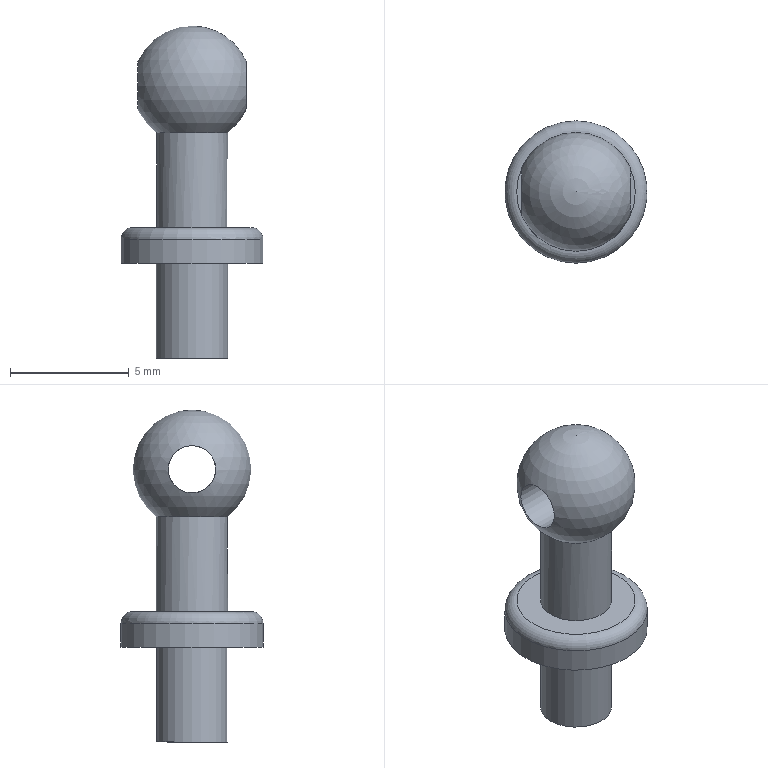Part | STEP file | 1-33.1 | 1 solid | 9 faces | box 6 x 6 x 14 mm | volume 146.542 mm3 | cylinder 4 | plane 3 | sphere 1 | torus 1 | commonest cylinder face diameters 3 x2 2 x1 6 x1
STEP:
#1=CARTESIAN_POINT('',(0.,0.,0.));
#2=DIRECTION('',(0.,0.,1.));
#3=DIRECTION('',(1.,0.,0.));
#4=AXIS2_PLACEMENT_3D('',#1,#2,#3);
#5=CARTESIAN_POINT('',(0.,1.5,-6.));
#6=VERTEX_POINT('',#5);
#7=CARTESIAN_POINT('',(0.,0.,-6.));
#8=DIRECTION('',(0.,0.,-1.));
#9=DIRECTION('',(0.,1.,0.));
#10=AXIS2_PLACEMENT_3D('',#7,#8,#9);
#11=CIRCLE('',#10,1.5);
#12=CARTESIAN_POINT('',(0.,0.,0.));
#13=DIRECTION('',(0.,0.,-1.));
#14=DIRECTION('',(0.,1.,0.));
#15=AXIS2_PLACEMENT_3D('',#12,#13,#14);
#16=CYLINDRICAL_SURFACE('',#15,1.5);
#17=CARTESIAN_POINT('',(0.,6.));
#18=DIRECTION('',(1.,0.));
#19=VECTOR('',#18,1.);
#20=LINE('',#17,#19);
#21=(GEOMETRIC_REPRESENTATION_CONTEXT(2)PARAMETRIC_REPRESENTATION_CONTEXT()REPRESENTATION_CONTEXT('',''));
#22=DEFINITIONAL_REPRESENTATION('',(#20),#21);
#23=PCURVE('',#16,#22);
#24=CARTESIAN_POINT('',(0.,-0.8038,-6.));
#25=DIRECTION('',(0.,0.,-1.));
#26=DIRECTION('',(0.,1.,0.));
#27=AXIS2_PLACEMENT_3D('',#24,#25,#26);
#28=PLANE('',#27);
#29=CARTESIAN_POINT('',(0.8038,0.));
#30=DIRECTION('',(1.,0.));
#31=AXIS2_PLACEMENT_2D('',#29,#30);
#32=CIRCLE('',#31,1.5);
#33=(GEOMETRIC_REPRESENTATION_CONTEXT(2)PARAMETRIC_REPRESENTATION_CONTEXT()REPRESENTATION_CONTEXT('',''));
#34=DEFINITIONAL_REPRESENTATION('',(#32),#33);
#35=PCURVE('',#28,#34);
#36=SURFACE_CURVE('',#11,(#23,#35),.PCURVE_S1.);
#37=EDGE_CURVE('',#6,#6,#36,.T.);
#38=ORIENTED_EDGE('',*,*,#37,.F.);
#39=CARTESIAN_POINT('',(0.,1.5,-2.));
#40=VERTEX_POINT('',#39);
#41=CARTESIAN_POINT('',(0.,1.5,-2.));
#42=DIRECTION('',(0.,0.,-1.));
#43=VECTOR('',#42,1.);
#44=LINE('',#41,#43);
#45=CARTESIAN_POINT('',(0.,2.));
#46=DIRECTION('',(0.,1.));
#47=VECTOR('',#46,1.);
#48=LINE('',#45,#47);
#49=(GEOMETRIC_REPRESENTATION_CONTEXT(2)PARAMETRIC_REPRESENTATION_CONTEXT()REPRESENTATION_CONTEXT('',''));
#50=DEFINITIONAL_REPRESENTATION('',(#48),#49);
#51=PCURVE('',#16,#50);
#52=CARTESIAN_POINT('',(6.283,2.));
#53=DIRECTION('',(0.,1.));
#54=VECTOR('',#53,1.);
#55=LINE('',#52,#54);
#56=(GEOMETRIC_REPRESENTATION_CONTEXT(2)PARAMETRIC_REPRESENTATION_CONTEXT()REPRESENTATION_CONTEXT('',''));
#57=DEFINITIONAL_REPRESENTATION('',(#55),#56);
#58=PCURVE('',#16,#57);
#59=SEAM_CURVE('',#44,(#51,#58),.PCURVE_S1.);
#60=EDGE_CURVE('',#40,#6,#59,.T.);
#61=ORIENTED_EDGE('',*,*,#60,.F.);
#62=CARTESIAN_POINT('',(1.5,0.,-2.));
#63=VERTEX_POINT('',#62);
#64=CARTESIAN_POINT('',(0.,0.,-2.));
#65=DIRECTION('',(0.,0.,-1.));
#66=DIRECTION('',(0.,1.,0.));
#67=AXIS2_PLACEMENT_3D('',#64,#65,#66);
#68=CIRCLE('',#67,1.5);
#69=CARTESIAN_POINT('',(0.,2.));
#70=DIRECTION('',(1.,0.));
#71=VECTOR('',#70,1.);
#72=LINE('',#69,#71);
#73=(GEOMETRIC_REPRESENTATION_CONTEXT(2)PARAMETRIC_REPRESENTATION_CONTEXT()REPRESENTATION_CONTEXT('',''));
#74=DEFINITIONAL_REPRESENTATION('',(#72),#73);
#75=PCURVE('',#16,#74);
#76=CARTESIAN_POINT('',(0.,0.,0.));
#77=DIRECTION('',(0.,0.,1.));
#78=DIRECTION('',(1.,0.,0.));
#79=AXIS2_PLACEMENT_3D('',#76,#77,#78);
#80=SPHERICAL_SURFACE('',#79,2.5);
#81=CARTESIAN_POINT('',(1.571,-0.9273));
#82=DIRECTION('',(-1.,0.));
#83=VECTOR('',#82,1.);
#84=LINE('',#81,#83);
#85=(GEOMETRIC_REPRESENTATION_CONTEXT(2)PARAMETRIC_REPRESENTATION_CONTEXT()REPRESENTATION_CONTEXT('',''));
#86=DEFINITIONAL_REPRESENTATION('',(#84),#85);
#87=PCURVE('',#80,#86);
#88=SURFACE_CURVE('',#68,(#75,#87),.PCURVE_S1.);
#89=EDGE_CURVE('',#40,#63,#88,.T.);
#90=ORIENTED_EDGE('',*,*,#89,.T.);
#91=CARTESIAN_POINT('',(0.,0.,-2.));
#92=DIRECTION('',(0.,0.,-1.));
#93=DIRECTION('',(1.,0.,0.));
#94=AXIS2_PLACEMENT_3D('',#91,#92,#93);
#95=CIRCLE('',#94,1.5);
#96=CARTESIAN_POINT('',(1.571,2.));
#97=DIRECTION('',(1.,0.));
#98=VECTOR('',#97,1.);
#99=LINE('',#96,#98);
#100=(GEOMETRIC_REPRESENTATION_CONTEXT(2)PARAMETRIC_REPRESENTATION_CONTEXT()REPRESENTATION_CONTEXT('',''));
#101=DEFINITIONAL_REPRESENTATION('',(#99),#100);
#102=PCURVE('',#16,#101);
#103=CARTESIAN_POINT('',(6.283,-0.9273));
#104=DIRECTION('',(-1.,0.));
#105=VECTOR('',#104,1.);
#106=LINE('',#103,#105);
#107=(GEOMETRIC_REPRESENTATION_CONTEXT(2)PARAMETRIC_REPRESENTATION_CONTEXT()REPRESENTATION_CONTEXT('',''));
#108=DEFINITIONAL_REPRESENTATION('',(#106),#107);
#109=PCURVE('',#80,#108);
#110=SURFACE_CURVE('',#95,(#102,#109),.PCURVE_S1.);
#111=EDGE_CURVE('',#63,#40,#110,.T.);
#112=ORIENTED_EDGE('',*,*,#111,.T.);
#113=ORIENTED_EDGE('',*,*,#60,.T.);
#114=EDGE_LOOP('',(#38,#61,#90,#112,#113));
#115=FACE_BOUND('',#114,.T.);
#116=ADVANCED_FACE('',(#115),#16,.T.);
#117=CARTESIAN_POINT('',(0.,3.,-7.5));
#118=VERTEX_POINT('',#117);
#119=CARTESIAN_POINT('',(0.,0.,-7.5));
#120=DIRECTION('',(0.,0.,-1.));
#121=DIRECTION('',(0.,1.,0.));
#122=AXIS2_PLACEMENT_3D('',#119,#120,#121);
#123=CIRCLE('',#122,3.);
#124=CARTESIAN_POINT('',(0.,-0.8038,-7.5));
#125=DIRECTION('',(0.,0.,-1.));
#126=DIRECTION('',(0.,1.,0.));
#127=AXIS2_PLACEMENT_3D('',#124,#125,#126);
#128=PLANE('',#127);
#129=CARTESIAN_POINT('',(0.8038,0.));
#130=DIRECTION('',(1.,0.));
#131=AXIS2_PLACEMENT_2D('',#129,#130);
#132=CIRCLE('',#131,3.);
#133=(GEOMETRIC_REPRESENTATION_CONTEXT(2)PARAMETRIC_REPRESENTATION_CONTEXT()REPRESENTATION_CONTEXT('',''));
#134=DEFINITIONAL_REPRESENTATION('',(#132),#133);
#135=PCURVE('',#128,#134);
#136=CARTESIAN_POINT('',(0.,0.,-6.));
#137=DIRECTION('',(0.,0.,-1.));
#138=DIRECTION('',(0.,1.,0.));
#139=AXIS2_PLACEMENT_3D('',#136,#137,#138);
#140=CYLINDRICAL_SURFACE('',#139,3.);
#141=CARTESIAN_POINT('',(0.,1.5));
#142=DIRECTION('',(1.,0.));
#143=VECTOR('',#142,1.);
#144=LINE('',#141,#143);
#145=(GEOMETRIC_REPRESENTATION_CONTEXT(2)PARAMETRIC_REPRESENTATION_CONTEXT()REPRESENTATION_CONTEXT('',''));
#146=DEFINITIONAL_REPRESENTATION('',(#144),#145);
#147=PCURVE('',#140,#146);
#148=SURFACE_CURVE('',#123,(#135,#147),.PCURVE_S1.);
#149=EDGE_CURVE('',#118,#118,#148,.T.);
#150=ORIENTED_EDGE('',*,*,#149,.T.);
#151=EDGE_LOOP('',(#150));
#152=FACE_BOUND('',#151,.T.);
#153=CARTESIAN_POINT('',(1.5,0.,-7.5));
#154=VERTEX_POINT('',#153);
#155=CARTESIAN_POINT('',(0.,0.,-7.5));
#156=DIRECTION('',(0.,0.,-1.));
#157=DIRECTION('',(1.,0.,0.));
#158=AXIS2_PLACEMENT_3D('',#155,#156,#157);
#159=CIRCLE('',#158,1.5);
#160=CARTESIAN_POINT('',(0.8038,0.));
#161=DIRECTION('',(0.,1.));
#162=AXIS2_PLACEMENT_2D('',#160,#161);
#163=CIRCLE('',#162,1.5);
#164=(GEOMETRIC_REPRESENTATION_CONTEXT(2)PARAMETRIC_REPRESENTATION_CONTEXT()REPRESENTATION_CONTEXT('',''));
#165=DEFINITIONAL_REPRESENTATION('',(#163),#164);
#166=PCURVE('',#128,#165);
#167=CARTESIAN_POINT('',(0.,0.,-7.5));
#168=DIRECTION('',(0.,0.,-1.));
#169=DIRECTION('',(1.,0.,0.));
#170=AXIS2_PLACEMENT_3D('',#167,#168,#169);
#171=CYLINDRICAL_SURFACE('',#170,1.5);
#172=CARTESIAN_POINT('',(0.,0.));
#173=DIRECTION('',(1.,0.));
#174=VECTOR('',#173,1.);
#175=LINE('',#172,#174);
#176=(GEOMETRIC_REPRESENTATION_CONTEXT(2)PARAMETRIC_REPRESENTATION_CONTEXT()REPRESENTATION_CONTEXT('',''));
#177=DEFINITIONAL_REPRESENTATION('',(#175),#176);
#178=PCURVE('',#171,#177);
#179=SURFACE_CURVE('',#159,(#166,#178),.PCURVE_S1.);
#180=EDGE_CURVE('',#154,#154,#179,.T.);
#181=ORIENTED_EDGE('',*,*,#180,.F.);
#182=EDGE_LOOP('',(#181));
#183=FACE_BOUND('',#182,.T.);
#184=ADVANCED_FACE('',(#152,#183),#128,.T.);
#185=ORIENTED_EDGE('',*,*,#180,.T.);
#186=CARTESIAN_POINT('',(1.5,0.,-11.5));
#187=VERTEX_POINT('',#186);
#188=CARTESIAN_POINT('',(1.5,0.,-7.5));
#189=DIRECTION('',(0.,0.,-1.));
#190=VECTOR('',#189,1.);
#191=LINE('',#188,#190);
#192=CARTESIAN_POINT('',(6.283,0.));
#193=DIRECTION('',(0.,1.));
#194=VECTOR('',#193,1.);
#195=LINE('',#192,#194);
#196=(GEOMETRIC_REPRESENTATION_CONTEXT(2)PARAMETRIC_REPRESENTATION_CONTEXT()REPRESENTATION_CONTEXT('',''));
#197=DEFINITIONAL_REPRESENTATION('',(#195),#196);
#198=PCURVE('',#171,#197);
#199=CARTESIAN_POINT('',(0.,0.));
#200=DIRECTION('',(0.,1.));
#201=VECTOR('',#200,1.);
#202=LINE('',#199,#201);
#203=(GEOMETRIC_REPRESENTATION_CONTEXT(2)PARAMETRIC_REPRESENTATION_CONTEXT()REPRESENTATION_CONTEXT('',''));
#204=DEFINITIONAL_REPRESENTATION('',(#202),#203);
#205=PCURVE('',#171,#204);
#206=SEAM_CURVE('',#191,(#198,#205),.PCURVE_S1.);
#207=EDGE_CURVE('',#154,#187,#206,.T.);
#208=ORIENTED_EDGE('',*,*,#207,.T.);
#209=CARTESIAN_POINT('',(0.,0.,-11.5));
#210=DIRECTION('',(0.,0.,-1.));
#211=DIRECTION('',(1.,0.,0.));
#212=AXIS2_PLACEMENT_3D('',#209,#210,#211);
#213=CIRCLE('',#212,1.5);
#214=CARTESIAN_POINT('',(0.,4.));
#215=DIRECTION('',(1.,0.));
#216=VECTOR('',#215,1.);
#217=LINE('',#214,#216);
#218=(GEOMETRIC_REPRESENTATION_CONTEXT(2)PARAMETRIC_REPRESENTATION_CONTEXT()REPRESENTATION_CONTEXT('',''));
#219=DEFINITIONAL_REPRESENTATION('',(#217),#218);
#220=PCURVE('',#171,#219);
#221=CARTESIAN_POINT('',(-0.4019,0.,-11.5));
#222=DIRECTION('',(0.,0.,-1.));
#223=DIRECTION('',(1.,0.,0.));
#224=AXIS2_PLACEMENT_3D('',#221,#222,#223);
#225=PLANE('',#224);
#226=CARTESIAN_POINT('',(0.4019,0.));
#227=DIRECTION('',(1.,0.));
#228=AXIS2_PLACEMENT_2D('',#226,#227);
#229=CIRCLE('',#228,1.5);
#230=(GEOMETRIC_REPRESENTATION_CONTEXT(2)PARAMETRIC_REPRESENTATION_CONTEXT()REPRESENTATION_CONTEXT('',''));
#231=DEFINITIONAL_REPRESENTATION('',(#229),#230);
#232=PCURVE('',#225,#231);
#233=SURFACE_CURVE('',#213,(#220,#232),.PCURVE_S1.);
#234=EDGE_CURVE('',#187,#187,#233,.T.);
#235=ORIENTED_EDGE('',*,*,#234,.F.);
#236=ORIENTED_EDGE('',*,*,#207,.F.);
#237=EDGE_LOOP('',(#185,#208,#235,#236));
#238=FACE_BOUND('',#237,.T.);
#239=ADVANCED_FACE('',(#238),#171,.T.);
#240=ORIENTED_EDGE('',*,*,#234,.T.);
#241=EDGE_LOOP('',(#240));
#242=FACE_BOUND('',#241,.T.);
#243=ADVANCED_FACE('',(#242),#225,.T.);
#244=CARTESIAN_POINT('',(2.291,0.,1.));
#245=VERTEX_POINT('',#244);
#246=CARTESIAN_POINT('',(0.,0.,2.5));
#247=VERTEX_POINT('',#246);
#248=CARTESIAN_POINT('',(0.,0.,0.));
#249=DIRECTION('',(0.,-1.,0.));
#250=DIRECTION('',(0.9165,0.,0.4));
#251=AXIS2_PLACEMENT_3D('',#248,#249,#250);
#252=CIRCLE('',#251,2.5);
#253=CARTESIAN_POINT('',(0.,0.4115));
#254=CARTESIAN_POINT('',(0.,0.4291));
#255=CARTESIAN_POINT('',(0.,0.4642));
#256=CARTESIAN_POINT('',(0.,0.5169));
#257=CARTESIAN_POINT('',(0.,0.5696));
#258=CARTESIAN_POINT('',(0.,0.6223));
#259=CARTESIAN_POINT('',(0.,0.675));
#260=CARTESIAN_POINT('',(0.,0.7277));
#261=CARTESIAN_POINT('',(0.,0.7804));
#262=CARTESIAN_POINT('',(0.,0.8331));
#263=CARTESIAN_POINT('',(0.,0.8858));
#264=CARTESIAN_POINT('',(0.,0.9385));
#265=CARTESIAN_POINT('',(0.,0.9912));
#266=CARTESIAN_POINT('',(0.,1.044));
#267=CARTESIAN_POINT('',(0.,1.097));
#268=CARTESIAN_POINT('',(0.,1.149));
#269=CARTESIAN_POINT('',(0.,1.202));
#270=CARTESIAN_POINT('',(0.,1.255));
#271=CARTESIAN_POINT('',(0.,1.307));
#272=CARTESIAN_POINT('',(0.,1.36));
#273=CARTESIAN_POINT('',(0.,1.413));
#274=CARTESIAN_POINT('',(0.,1.465));
#275=CARTESIAN_POINT('',(0.,1.518));
#276=CARTESIAN_POINT('',(0.,1.553));
#277=CARTESIAN_POINT('',(0.,1.571));
#278=B_SPLINE_CURVE_WITH_KNOTS('',3,(#253,#254,#255,#256,#257,#258,#259,#260,#261,#262,#263,#264,#265,#266,#267,#268,#269,#270,#271,#272,#273,#274,#275,#276,#277),.UNSPECIFIED.,.F.,.F.,(4,1,1,1,1,1,1,1,1,1,1,1,1,1,1,1,1,1,1,1,1,1,4),(0.,0.05269,0.1054,0.1581,0.2108,0.2635,0.3162,0.3689,0.4216,0.4743,0.5269,0.5796,0.6323,0.685,0.7377,0.7904,0.8431,0.8958,0.9485,1.001,1.054,1.107,1.159),.QUASI_UNIFORM_KNOTS.);
#279=(GEOMETRIC_REPRESENTATION_CONTEXT(2)PARAMETRIC_REPRESENTATION_CONTEXT()REPRESENTATION_CONTEXT('',''));
#280=DEFINITIONAL_REPRESENTATION('',(#278),#279);
#281=PCURVE('',#80,#280);
#282=CARTESIAN_POINT('',(6.283,0.4115));
#283=CARTESIAN_POINT('',(6.283,0.4291));
#284=CARTESIAN_POINT('',(6.283,0.4642));
#285=CARTESIAN_POINT('',(6.283,0.5169));
#286=CARTESIAN_POINT('',(6.283,0.5696));
#287=CARTESIAN_POINT('',(6.283,0.6223));
#288=CARTESIAN_POINT('',(6.283,0.675));
#289=CARTESIAN_POINT('',(6.283,0.7277));
#290=CARTESIAN_POINT('',(6.283,0.7804));
#291=CARTESIAN_POINT('',(6.283,0.8331));
#292=CARTESIAN_POINT('',(6.283,0.8858));
#293=CARTESIAN_POINT('',(6.283,0.9385));
#294=CARTESIAN_POINT('',(6.283,0.9912));
#295=CARTESIAN_POINT('',(6.283,1.044));
#296=CARTESIAN_POINT('',(6.283,1.097));
#297=CARTESIAN_POINT('',(6.283,1.149));
#298=CARTESIAN_POINT('',(6.283,1.202));
#299=CARTESIAN_POINT('',(6.283,1.255));
#300=CARTESIAN_POINT('',(6.283,1.307));
#301=CARTESIAN_POINT('',(6.283,1.36));
#302=CARTESIAN_POINT('',(6.283,1.413));
#303=CARTESIAN_POINT('',(6.283,1.465));
#304=CARTESIAN_POINT('',(6.283,1.518));
#305=CARTESIAN_POINT('',(6.283,1.553));
#306=CARTESIAN_POINT('',(6.283,1.571));
#307=B_SPLINE_CURVE_WITH_KNOTS('',3,(#282,#283,#284,#285,#286,#287,#288,#289,#290,#291,#292,#293,#294,#295,#296,#297,#298,#299,#300,#301,#302,#303,#304,#305,#306),.UNSPECIFIED.,.F.,.F.,(4,1,1,1,1,1,1,1,1,1,1,1,1,1,1,1,1,1,1,1,1,1,4),(0.,0.05269,0.1054,0.1581,0.2108,0.2635,0.3162,0.3689,0.4216,0.4743,0.5269,0.5796,0.6323,0.685,0.7377,0.7904,0.8431,0.8958,0.9485,1.001,1.054,1.107,1.159),.QUASI_UNIFORM_KNOTS.);
#308=(GEOMETRIC_REPRESENTATION_CONTEXT(2)PARAMETRIC_REPRESENTATION_CONTEXT()REPRESENTATION_CONTEXT('',''));
#309=DEFINITIONAL_REPRESENTATION('',(#307),#308);
#310=PCURVE('',#80,#309);
#311=SEAM_CURVE('',#252,(#281,#310),.PCURVE_S1.);
#312=EDGE_CURVE('',#245,#247,#311,.T.);
#313=ORIENTED_EDGE('',*,*,#312,.F.);
#314=CARTESIAN_POINT('',(2.291,1.,0.));
#315=VERTEX_POINT('',#314);
#316=CARTESIAN_POINT('',(2.291,0.,0.));
#317=DIRECTION('',(1.,0.,0.));
#318=DIRECTION('',(0.,1.,0.));
#319=AXIS2_PLACEMENT_3D('',#316,#317,#318);
#320=CIRCLE('',#319,1.);
#321=CARTESIAN_POINT('',(0.4115,0.));
#322=CARTESIAN_POINT('',(0.4115,0.00952));
#323=CARTESIAN_POINT('',(0.4109,0.02856));
#324=CARTESIAN_POINT('',(0.4081,0.057));
#325=CARTESIAN_POINT('',(0.4034,0.08519));
#326=CARTESIAN_POINT('',(0.3969,0.113));
#327=CARTESIAN_POINT('',(0.3885,0.1403));
#328=CARTESIAN_POINT('',(0.3782,0.1671));
#329=CARTESIAN_POINT('',(0.3661,0.193));
#330=CARTESIAN_POINT('',(0.3522,0.2181));
#331=CARTESIAN_POINT('',(0.3364,0.2423));
#332=CARTESIAN_POINT('',(0.3189,0.2652));
#333=CARTESIAN_POINT('',(0.2996,0.287));
#334=CARTESIAN_POINT('',(0.2787,0.3074));
#335=CARTESIAN_POINT('',(0.2561,0.3262));
#336=CARTESIAN_POINT('',(0.232,0.3435));
#337=CARTESIAN_POINT('',(0.2064,0.359));
#338=CARTESIAN_POINT('',(0.1795,0.3727));
#339=CARTESIAN_POINT('',(0.1515,0.3845));
#340=CARTESIAN_POINT('',(0.1225,0.3943));
#341=CARTESIAN_POINT('',(0.09261,0.4019));
#342=CARTESIAN_POINT('',(0.0621,0.4074));
#343=CARTESIAN_POINT('',(0.03116,0.4108));
#344=CARTESIAN_POINT('',(0.01039,0.4115));
#345=CARTESIAN_POINT('',(0.,0.4115));
#346=B_SPLINE_CURVE_WITH_KNOTS('',3,(#321,#322,#323,#324,#325,#326,#327,#328,#329,#330,#331,#332,#333,#334,#335,#336,#337,#338,#339,#340,#341,#342,#343,#344,#345),.UNSPECIFIED.,.F.,.F.,(4,1,1,1,1,1,1,1,1,1,1,1,1,1,1,1,1,1,1,1,1,1,4),(0.,0.0714,0.1428,0.2142,0.2856,0.357,0.4284,0.4998,0.5712,0.6426,0.714,0.7854,0.8568,0.9282,0.9996,1.071,1.142,1.214,1.285,1.357,1.428,1.499,1.571),.QUASI_UNIFORM_KNOTS.);
#347=(GEOMETRIC_REPRESENTATION_CONTEXT(2)PARAMETRIC_REPRESENTATION_CONTEXT()REPRESENTATION_CONTEXT('',''));
#348=DEFINITIONAL_REPRESENTATION('',(#346),#347);
#349=PCURVE('',#80,#348);
#350=CARTESIAN_POINT('',(-4.,0.,0.));
#351=DIRECTION('',(1.,0.,0.));
#352=DIRECTION('',(0.,1.,0.));
#353=AXIS2_PLACEMENT_3D('',#350,#351,#352);
#354=CYLINDRICAL_SURFACE('',#353,1.);
#355=CARTESIAN_POINT('',(0.,6.291));
#356=DIRECTION('',(1.,0.));
#357=VECTOR('',#356,1.);
#358=LINE('',#355,#357);
#359=(GEOMETRIC_REPRESENTATION_CONTEXT(2)PARAMETRIC_REPRESENTATION_CONTEXT()REPRESENTATION_CONTEXT('',''));
#360=DEFINITIONAL_REPRESENTATION('',(#358),#359);
#361=PCURVE('',#354,#360);
#362=SURFACE_CURVE('',#320,(#349,#361),.PCURVE_S1.);
#363=EDGE_CURVE('',#315,#245,#362,.T.);
#364=ORIENTED_EDGE('',*,*,#363,.F.);
#365=CARTESIAN_POINT('',(2.291,0.,-1.));
#366=VERTEX_POINT('',#365);
#367=CARTESIAN_POINT('',(2.291,0.,0.));
#368=DIRECTION('',(1.,0.,0.));
#369=DIRECTION('',(0.,0.,-1.));
#370=AXIS2_PLACEMENT_3D('',#367,#368,#369);
#371=CIRCLE('',#370,1.);
#372=CARTESIAN_POINT('',(0.,-0.4115));
#373=CARTESIAN_POINT('',(0.01039,-0.4115));
#374=CARTESIAN_POINT('',(0.03116,-0.4108));
#375=CARTESIAN_POINT('',(0.0621,-0.4074));
#376=CARTESIAN_POINT('',(0.09261,-0.4019));
#377=CARTESIAN_POINT('',(0.1225,-0.3943));
#378=CARTESIAN_POINT('',(0.1515,-0.3845));
#379=CARTESIAN_POINT('',(0.1795,-0.3727));
#380=CARTESIAN_POINT('',(0.2064,-0.359));
#381=CARTESIAN_POINT('',(0.232,-0.3435));
#382=CARTESIAN_POINT('',(0.2561,-0.3262));
#383=CARTESIAN_POINT('',(0.2787,-0.3074));
#384=CARTESIAN_POINT('',(0.2996,-0.287));
#385=CARTESIAN_POINT('',(0.3189,-0.2652));
#386=CARTESIAN_POINT('',(0.3364,-0.2423));
#387=CARTESIAN_POINT('',(0.3522,-0.2181));
#388=CARTESIAN_POINT('',(0.3661,-0.193));
#389=CARTESIAN_POINT('',(0.3782,-0.1671));
#390=CARTESIAN_POINT('',(0.3885,-0.1403));
#391=CARTESIAN_POINT('',(0.3969,-0.113));
#392=CARTESIAN_POINT('',(0.4034,-0.08519));
#393=CARTESIAN_POINT('',(0.4081,-0.057));
#394=CARTESIAN_POINT('',(0.4109,-0.02856));
#395=CARTESIAN_POINT('',(0.4115,-0.00952));
#396=CARTESIAN_POINT('',(0.4115,0.));
#397=B_SPLINE_CURVE_WITH_KNOTS('',3,(#372,#373,#374,#375,#376,#377,#378,#379,#380,#381,#382,#383,#384,#385,#386,#387,#388,#389,#390,#391,#392,#393,#394,#395,#396),.UNSPECIFIED.,.F.,.F.,(4,1,1,1,1,1,1,1,1,1,1,1,1,1,1,1,1,1,1,1,1,1,4),(0.,0.0714,0.1428,0.2142,0.2856,0.357,0.4284,0.4998,0.5712,0.6426,0.714,0.7854,0.8568,0.9282,0.9996,1.071,1.142,1.214,1.285,1.357,1.428,1.499,1.571),.QUASI_UNIFORM_KNOTS.);
#398=(GEOMETRIC_REPRESENTATION_CONTEXT(2)PARAMETRIC_REPRESENTATION_CONTEXT()REPRESENTATION_CONTEXT('',''));
#399=DEFINITIONAL_REPRESENTATION('',(#397),#398);
#400=PCURVE('',#80,#399);
#401=CARTESIAN_POINT('',(4.712,6.291));
#402=DIRECTION('',(1.,0.));
#403=VECTOR('',#402,1.);
#404=LINE('',#401,#403);
#405=(GEOMETRIC_REPRESENTATION_CONTEXT(2)PARAMETRIC_REPRESENTATION_CONTEXT()REPRESENTATION_CONTEXT('',''));
#406=DEFINITIONAL_REPRESENTATION('',(#404),#405);
#407=PCURVE('',#354,#406);
#408=SURFACE_CURVE('',#371,(#400,#407),.PCURVE_S1.);
#409=EDGE_CURVE('',#366,#315,#408,.T.);
#410=ORIENTED_EDGE('',*,*,#409,.F.);
#411=CARTESIAN_POINT('',(0.,0.,0.));
#412=DIRECTION('',(0.,-1.,0.));
#413=DIRECTION('',(0.6,0.,-0.8));
#414=AXIS2_PLACEMENT_3D('',#411,#412,#413);
#415=CIRCLE('',#414,2.5);
#416=CARTESIAN_POINT('',(0.,-0.9273));
#417=DIRECTION('',(0.,1.));
#418=VECTOR('',#417,1.);
#419=LINE('',#416,#418);
#420=(GEOMETRIC_REPRESENTATION_CONTEXT(2)PARAMETRIC_REPRESENTATION_CONTEXT()REPRESENTATION_CONTEXT('',''));
#421=DEFINITIONAL_REPRESENTATION('',(#419),#420);
#422=PCURVE('',#80,#421);
#423=CARTESIAN_POINT('',(6.283,-0.9273));
#424=DIRECTION('',(0.,1.));
#425=VECTOR('',#424,1.);
#426=LINE('',#423,#425);
#427=(GEOMETRIC_REPRESENTATION_CONTEXT(2)PARAMETRIC_REPRESENTATION_CONTEXT()REPRESENTATION_CONTEXT('',''));
#428=DEFINITIONAL_REPRESENTATION('',(#426),#427);
#429=PCURVE('',#80,#428);
#430=SEAM_CURVE('',#415,(#422,#429),.PCURVE_S1.);
#431=EDGE_CURVE('',#63,#366,#430,.T.);
#432=ORIENTED_EDGE('',*,*,#431,.F.);
#433=ORIENTED_EDGE('',*,*,#89,.F.);
#434=ORIENTED_EDGE('',*,*,#111,.F.);
#435=ORIENTED_EDGE('',*,*,#431,.T.);
#436=CARTESIAN_POINT('',(2.291,0.,0.));
#437=DIRECTION('',(1.,0.,0.));
#438=DIRECTION('',(0.,0.,1.));
#439=AXIS2_PLACEMENT_3D('',#436,#437,#438);
#440=CIRCLE('',#439,1.);
#441=CARTESIAN_POINT('',(6.283,0.4115));
#442=CARTESIAN_POINT('',(6.262,0.4115));
#443=CARTESIAN_POINT('',(6.221,0.4085));
#444=CARTESIAN_POINT('',(6.16,0.3953));
#445=CARTESIAN_POINT('',(6.103,0.3737));
#446=CARTESIAN_POINT('',(6.051,0.3444));
#447=CARTESIAN_POINT('',(6.004,0.3081));
#448=CARTESIAN_POINT('',(5.963,0.2659));
#449=CARTESIAN_POINT('',(5.93,0.2186));
#450=CARTESIAN_POINT('',(5.904,0.1674));
#451=CARTESIAN_POINT('',(5.885,0.1133));
#452=CARTESIAN_POINT('',(5.874,0.05712));
#453=CARTESIAN_POINT('',(5.87,0.));
#454=CARTESIAN_POINT('',(5.874,-0.05712));
#455=CARTESIAN_POINT('',(5.885,-0.1133));
#456=CARTESIAN_POINT('',(5.904,-0.1674));
#457=CARTESIAN_POINT('',(5.93,-0.2186));
#458=CARTESIAN_POINT('',(5.963,-0.2659));
#459=CARTESIAN_POINT('',(6.004,-0.3081));
#460=CARTESIAN_POINT('',(6.051,-0.3444));
#461=CARTESIAN_POINT('',(6.103,-0.3737));
#462=CARTESIAN_POINT('',(6.16,-0.3953));
#463=CARTESIAN_POINT('',(6.221,-0.4085));
#464=CARTESIAN_POINT('',(6.262,-0.4115));
#465=CARTESIAN_POINT('',(6.283,-0.4115));
#466=B_SPLINE_CURVE_WITH_KNOTS('',3,(#441,#442,#443,#444,#445,#446,#447,#448,#449,#450,#451,#452,#453,#454,#455,#456,#457,#458,#459,#460,#461,#462,#463,#464,#465),.UNSPECIFIED.,.F.,.F.,(4,1,1,1,1,1,1,1,1,1,1,1,1,1,1,1,1,1,1,1,1,1,4),(0.,0.1428,0.2856,0.4284,0.5712,0.714,0.8568,0.9996,1.142,1.285,1.428,1.571,1.714,1.856,1.999,2.142,2.285,2.428,2.57,2.713,2.856,2.999,3.142),.QUASI_UNIFORM_KNOTS.);
#467=(GEOMETRIC_REPRESENTATION_CONTEXT(2)PARAMETRIC_REPRESENTATION_CONTEXT()REPRESENTATION_CONTEXT('',''));
#468=DEFINITIONAL_REPRESENTATION('',(#466),#467);
#469=PCURVE('',#80,#468);
#470=CARTESIAN_POINT('',(1.571,6.291));
#471=DIRECTION('',(1.,0.));
#472=VECTOR('',#471,1.);
#473=LINE('',#470,#472);
#474=(GEOMETRIC_REPRESENTATION_CONTEXT(2)PARAMETRIC_REPRESENTATION_CONTEXT()REPRESENTATION_CONTEXT('',''));
#475=DEFINITIONAL_REPRESENTATION('',(#473),#474);
#476=PCURVE('',#354,#475);
#477=SURFACE_CURVE('',#440,(#469,#476),.PCURVE_S1.);
#478=EDGE_CURVE('',#245,#366,#477,.T.);
#479=ORIENTED_EDGE('',*,*,#478,.F.);
#480=ORIENTED_EDGE('',*,*,#312,.T.);
#481=EDGE_LOOP('',(#313,#364,#410,#432,#433,#434,#435,#479,#480));
#482=FACE_BOUND('',#481,.T.);
#483=CARTESIAN_POINT('',(-2.291,1.,0.));
#484=VERTEX_POINT('',#483);
#485=CARTESIAN_POINT('',(-2.291,0.,0.));
#486=DIRECTION('',(-1.,0.,0.));
#487=DIRECTION('',(0.,1.,0.));
#488=AXIS2_PLACEMENT_3D('',#485,#486,#487);
#489=CIRCLE('',#488,1.);
#490=CARTESIAN_POINT('',(2.73,0.));
#491=CARTESIAN_POINT('',(2.73,-0.03807));
#492=CARTESIAN_POINT('',(2.74,-0.1142));
#493=CARTESIAN_POINT('',(2.785,-0.2206));
#494=CARTESIAN_POINT('',(2.859,-0.3111));
#495=CARTESIAN_POINT('',(2.959,-0.3776));
#496=CARTESIAN_POINT('',(3.078,-0.413));
#497=CARTESIAN_POINT('',(3.205,-0.413));
#498=CARTESIAN_POINT('',(3.324,-0.3776));
#499=CARTESIAN_POINT('',(3.424,-0.3111));
#500=CARTESIAN_POINT('',(3.498,-0.2206));
#501=CARTESIAN_POINT('',(3.543,-0.1142));
#502=CARTESIAN_POINT('',(3.558,0.));
#503=CARTESIAN_POINT('',(3.543,0.1142));
#504=CARTESIAN_POINT('',(3.498,0.2206));
#505=CARTESIAN_POINT('',(3.424,0.3111));
#506=CARTESIAN_POINT('',(3.324,0.3776));
#507=CARTESIAN_POINT('',(3.205,0.413));
#508=CARTESIAN_POINT('',(3.078,0.413));
#509=CARTESIAN_POINT('',(2.959,0.3776));
#510=CARTESIAN_POINT('',(2.859,0.3111));
#511=CARTESIAN_POINT('',(2.785,0.2206));
#512=CARTESIAN_POINT('',(2.74,0.1142));
#513=CARTESIAN_POINT('',(2.73,0.03807));
#514=CARTESIAN_POINT('',(2.73,0.));
#515=B_SPLINE_CURVE_WITH_KNOTS('',3,(#490,#491,#492,#493,#494,#495,#496,#497,#498,#499,#500,#501,#502,#503,#504,#505,#506,#507,#508,#509,#510,#511,#512,#513,#514),.UNSPECIFIED.,.F.,.F.,(4,1,1,1,1,1,1,1,1,1,1,1,1,1,1,1,1,1,1,1,1,1,4),(0.,0.2856,0.5712,0.8568,1.142,1.428,1.714,1.999,2.285,2.57,2.856,3.142,3.427,3.713,3.998,4.284,4.57,4.855,5.141,5.426,5.712,5.998,6.283),.QUASI_UNIFORM_KNOTS.);
#516=(GEOMETRIC_REPRESENTATION_CONTEXT(2)PARAMETRIC_REPRESENTATION_CONTEXT()REPRESENTATION_CONTEXT('',''));
#517=DEFINITIONAL_REPRESENTATION('',(#515),#516);
#518=PCURVE('',#80,#517);
#519=CARTESIAN_POINT('',(6.283,1.709));
#520=DIRECTION('',(-1.,0.));
#521=VECTOR('',#520,1.);
#522=LINE('',#519,#521);
#523=(GEOMETRIC_REPRESENTATION_CONTEXT(2)PARAMETRIC_REPRESENTATION_CONTEXT()REPRESENTATION_CONTEXT('',''));
#524=DEFINITIONAL_REPRESENTATION('',(#522),#523);
#525=PCURVE('',#354,#524);
#526=SURFACE_CURVE('',#489,(#518,#525),.PCURVE_S1.);
#527=EDGE_CURVE('',#484,#484,#526,.T.);
#528=ORIENTED_EDGE('',*,*,#527,.F.);
#529=EDGE_LOOP('',(#528));
#530=FACE_BOUND('',#529,.T.);
#531=ADVANCED_FACE('',(#482,#530),#80,.T.);
#532=CARTESIAN_POINT('',(-2.291,1.,0.));
#533=DIRECTION('',(1.,0.,0.));
#534=VECTOR('',#533,1.);
#535=LINE('',#532,#534);
#536=CARTESIAN_POINT('',(6.283,1.709));
#537=DIRECTION('',(0.,1.));
#538=VECTOR('',#537,1.);
#539=LINE('',#536,#538);
#540=(GEOMETRIC_REPRESENTATION_CONTEXT(2)PARAMETRIC_REPRESENTATION_CONTEXT()REPRESENTATION_CONTEXT('',''));
#541=DEFINITIONAL_REPRESENTATION('',(#539),#540);
#542=PCURVE('',#354,#541);
#543=CARTESIAN_POINT('',(0.,1.709));
#544=DIRECTION('',(0.,1.));
#545=VECTOR('',#544,1.);
#546=LINE('',#543,#545);
#547=(GEOMETRIC_REPRESENTATION_CONTEXT(2)PARAMETRIC_REPRESENTATION_CONTEXT()REPRESENTATION_CONTEXT('',''));
#548=DEFINITIONAL_REPRESENTATION('',(#546),#547);
#549=PCURVE('',#354,#548);
#550=SEAM_CURVE('',#535,(#542,#549),.PCURVE_S1.);
#551=EDGE_CURVE('',#484,#315,#550,.T.);
#552=ORIENTED_EDGE('',*,*,#551,.T.);
#553=ORIENTED_EDGE('',*,*,#409,.F.);
#554=ORIENTED_EDGE('',*,*,#478,.F.);
#555=ORIENTED_EDGE('',*,*,#363,.F.);
#556=ORIENTED_EDGE('',*,*,#551,.F.);
#557=ORIENTED_EDGE('',*,*,#527,.F.);
#558=EDGE_LOOP('',(#552,#553,#554,#555,#556,#557));
#559=FACE_BOUND('',#558,.F.);
#560=ADVANCED_FACE('',(#559),#354,.F.);
#561=CARTESIAN_POINT('',(0.,2.5,-6.));
#562=VERTEX_POINT('',#561);
#563=CARTESIAN_POINT('',(0.,0.,-6.));
#564=DIRECTION('',(0.,0.,1.));
#565=DIRECTION('',(0.,1.,0.));
#566=AXIS2_PLACEMENT_3D('',#563,#564,#565);
#567=CIRCLE('',#566,2.5);
#568=CARTESIAN_POINT('',(3.304,0.));
#569=CARTESIAN_POINT('',(3.304,-4.33));
#570=CARTESIAN_POINT('',(-0.4462,-2.165));
#571=CARTESIAN_POINT('',(-4.196,0.));
#572=CARTESIAN_POINT('',(-0.4462,2.165));
#573=CARTESIAN_POINT('',(3.304,4.33));
#574=CARTESIAN_POINT('',(3.304,0.));
#575=(BOUNDED_CURVE()B_SPLINE_CURVE(2,(#568,#569,#570,#571,#572,#573,#574),.UNSPECIFIED.,.T.,.F.)B_SPLINE_CURVE_WITH_KNOTS((1,2,2,2,2,1),(-2.094,0.,2.094,4.189,6.283,8.378),.UNSPECIFIED.)CURVE()GEOMETRIC_REPRESENTATION_ITEM()RATIONAL_B_SPLINE_CURVE((1.,0.5,1.,0.5,1.,0.5,1.))REPRESENTATION_ITEM(''));
#576=(GEOMETRIC_REPRESENTATION_CONTEXT(2)PARAMETRIC_REPRESENTATION_CONTEXT()REPRESENTATION_CONTEXT('',''));
#577=DEFINITIONAL_REPRESENTATION('',(#575),#576);
#578=PCURVE('',#28,#577);
#579=CARTESIAN_POINT('',(0.,0.,-6.5));
#580=DIRECTION('',(0.,0.,-1.));
#581=DIRECTION('',(0.,1.,0.));
#582=AXIS2_PLACEMENT_3D('',#579,#580,#581);
#583=TOROIDAL_SURFACE('',#582,2.5,0.5);
#584=CARTESIAN_POINT('',(6.283,4.712));
#585=DIRECTION('',(-1.,0.));
#586=VECTOR('',#585,1.);
#587=LINE('',#584,#586);
#588=(GEOMETRIC_REPRESENTATION_CONTEXT(2)PARAMETRIC_REPRESENTATION_CONTEXT()REPRESENTATION_CONTEXT('',''));
#589=DEFINITIONAL_REPRESENTATION('',(#587),#588);
#590=PCURVE('',#583,#589);
#591=SURFACE_CURVE('',#567,(#578,#590),.PCURVE_S1.);
#592=EDGE_CURVE('',#562,#562,#591,.T.);
#593=ORIENTED_EDGE('',*,*,#592,.F.);
#594=EDGE_LOOP('',(#593));
#595=FACE_BOUND('',#594,.F.);
#596=ORIENTED_EDGE('',*,*,#37,.F.);
#597=EDGE_LOOP('',(#596));
#598=FACE_BOUND('',#597,.F.);
#599=ADVANCED_FACE('',(#595,#598),#28,.F.);
#600=ORIENTED_EDGE('',*,*,#149,.F.);
#601=CARTESIAN_POINT('',(0.,3.,-6.5));
#602=VERTEX_POINT('',#601);
#603=CARTESIAN_POINT('',(0.,3.,-6.5));
#604=DIRECTION('',(0.,0.,-1.));
#605=VECTOR('',#604,1.);
#606=LINE('',#603,#605);
#607=CARTESIAN_POINT('',(0.,0.5));
#608=DIRECTION('',(0.,1.));
#609=VECTOR('',#608,1.);
#610=LINE('',#607,#609);
#611=(GEOMETRIC_REPRESENTATION_CONTEXT(2)PARAMETRIC_REPRESENTATION_CONTEXT()REPRESENTATION_CONTEXT('',''));
#612=DEFINITIONAL_REPRESENTATION('',(#610),#611);
#613=PCURVE('',#140,#612);
#614=CARTESIAN_POINT('',(6.283,0.5));
#615=DIRECTION('',(0.,1.));
#616=VECTOR('',#615,1.);
#617=LINE('',#614,#616);
#618=(GEOMETRIC_REPRESENTATION_CONTEXT(2)PARAMETRIC_REPRESENTATION_CONTEXT()REPRESENTATION_CONTEXT('',''));
#619=DEFINITIONAL_REPRESENTATION('',(#617),#618);
#620=PCURVE('',#140,#619);
#621=SEAM_CURVE('',#606,(#613,#620),.PCURVE_S1.);
#622=EDGE_CURVE('',#602,#118,#621,.T.);
#623=ORIENTED_EDGE('',*,*,#622,.F.);
#624=CARTESIAN_POINT('',(0.,0.,-6.5));
#625=DIRECTION('',(0.,0.,1.));
#626=DIRECTION('',(0.,1.,0.));
#627=AXIS2_PLACEMENT_3D('',#624,#625,#626);
#628=CIRCLE('',#627,3.);
#629=CARTESIAN_POINT('',(6.283,0.5));
#630=DIRECTION('',(-1.,0.));
#631=VECTOR('',#630,1.);
#632=LINE('',#629,#631);
#633=(GEOMETRIC_REPRESENTATION_CONTEXT(2)PARAMETRIC_REPRESENTATION_CONTEXT()REPRESENTATION_CONTEXT('',''));
#634=DEFINITIONAL_REPRESENTATION('',(#632),#633);
#635=PCURVE('',#140,#634);
#636=CARTESIAN_POINT('',(6.283,6.283));
#637=DIRECTION('',(-1.,0.));
#638=VECTOR('',#637,1.);
#639=LINE('',#636,#638);
#640=(GEOMETRIC_REPRESENTATION_CONTEXT(2)PARAMETRIC_REPRESENTATION_CONTEXT()REPRESENTATION_CONTEXT('',''));
#641=DEFINITIONAL_REPRESENTATION('',(#639),#640);
#642=PCURVE('',#583,#641);
#643=SURFACE_CURVE('',#628,(#635,#642),.PCURVE_S1.);
#644=EDGE_CURVE('',#602,#602,#643,.T.);
#645=ORIENTED_EDGE('',*,*,#644,.F.);
#646=ORIENTED_EDGE('',*,*,#622,.T.);
#647=EDGE_LOOP('',(#600,#623,#645,#646));
#648=FACE_BOUND('',#647,.T.);
#649=ADVANCED_FACE('',(#648),#140,.T.);
#650=ORIENTED_EDGE('',*,*,#592,.F.);
#651=CARTESIAN_POINT('',(0.,2.5,-6.5));
#652=DIRECTION('',(-1.,0.,0.));
#653=DIRECTION('',(0.,0.,1.));
#654=AXIS2_PLACEMENT_3D('',#651,#652,#653);
#655=CIRCLE('',#654,0.5);
#656=CARTESIAN_POINT('',(6.283,4.712));
#657=DIRECTION('',(0.,1.));
#658=VECTOR('',#657,1.);
#659=LINE('',#656,#658);
#660=(GEOMETRIC_REPRESENTATION_CONTEXT(2)PARAMETRIC_REPRESENTATION_CONTEXT()REPRESENTATION_CONTEXT('',''));
#661=DEFINITIONAL_REPRESENTATION('',(#659),#660);
#662=PCURVE('',#583,#661);
#663=CARTESIAN_POINT('',(0.,4.712));
#664=DIRECTION('',(0.,1.));
#665=VECTOR('',#664,1.);
#666=LINE('',#663,#665);
#667=(GEOMETRIC_REPRESENTATION_CONTEXT(2)PARAMETRIC_REPRESENTATION_CONTEXT()REPRESENTATION_CONTEXT('',''));
#668=DEFINITIONAL_REPRESENTATION('',(#666),#667);
#669=PCURVE('',#583,#668);
#670=SEAM_CURVE('',#655,(#662,#669),.PCURVE_S1.);
#671=EDGE_CURVE('',#562,#602,#670,.T.);
#672=ORIENTED_EDGE('',*,*,#671,.T.);
#673=ORIENTED_EDGE('',*,*,#644,.T.);
#674=ORIENTED_EDGE('',*,*,#671,.F.);
#675=EDGE_LOOP('',(#650,#672,#673,#674));
#676=FACE_BOUND('',#675,.T.);
#677=ADVANCED_FACE('',(#676),#583,.T.);
#678=CLOSED_SHELL('',(#116,#184,#239,#243,#531,#560,#599,#649,#677));
#679=MANIFOLD_SOLID_BREP('',#678);
#680=(LENGTH_UNIT()NAMED_UNIT(*)SI_UNIT(.MILLI.,.METRE.));
#681=UNCERTAINTY_MEASURE_WITH_UNIT(LENGTH_MEASURE(0.0000001),#680,'','');
#682=(NAMED_UNIT(*)PLANE_ANGLE_UNIT()SI_UNIT($,.RADIAN.));
#683=(NAMED_UNIT(*)SI_UNIT($,.STERADIAN.)SOLID_ANGLE_UNIT());
#684=(GEOMETRIC_REPRESENTATION_CONTEXT(3)GLOBAL_UNCERTAINTY_ASSIGNED_CONTEXT((#681))GLOBAL_UNIT_ASSIGNED_CONTEXT((#680,#682,#683))REPRESENTATION_CONTEXT('',''));
#685=ADVANCED_BREP_SHAPE_REPRESENTATION('',(#4,#679),#684);